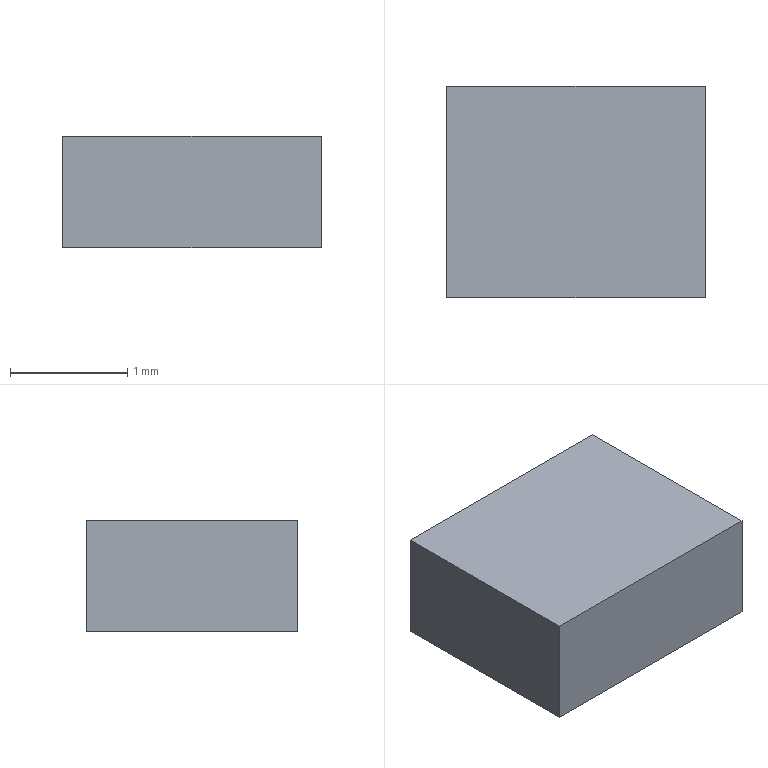Part | Creo | 1 solid | 6 faces | box 2.2 x 1.8 x 0.95 mm | volume 3.762 mm3 | plane 6
STEP:
#1=CARTESIAN_POINT('',(0.,0.,0.));
#2=DIRECTION('',(0.,0.,1.));
#3=DIRECTION('',(1.,0.,0.));
#4=AXIS2_PLACEMENT_3D('',#1,#2,#3);
#5=CARTESIAN_POINT('',(-1.1,0.9,0.));
#6=VERTEX_POINT('',#5);
#7=CARTESIAN_POINT('',(-1.1,-0.9,0.));
#8=VERTEX_POINT('',#7);
#9=CARTESIAN_POINT('',(-1.1,0.9,0.));
#10=DIRECTION('',(0.,-1.,0.));
#11=VECTOR('',#10,1.8);
#12=LINE('',#9,#11);
#13=EDGE_CURVE('',#6,#8,#12,.T.);
#14=ORIENTED_EDGE('',*,*,#13,.T.);
#15=CARTESIAN_POINT('',(1.1,-0.9,0.));
#16=VERTEX_POINT('',#15);
#17=CARTESIAN_POINT('',(-1.1,-0.9,0.));
#18=DIRECTION('',(1.,0.,0.));
#19=VECTOR('',#18,2.2);
#20=LINE('',#17,#19);
#21=EDGE_CURVE('',#8,#16,#20,.T.);
#22=ORIENTED_EDGE('',*,*,#21,.T.);
#23=CARTESIAN_POINT('',(1.1,0.9,0.));
#24=VERTEX_POINT('',#23);
#25=CARTESIAN_POINT('',(1.1,-0.9,0.));
#26=DIRECTION('',(0.,1.,0.));
#27=VECTOR('',#26,1.8);
#28=LINE('',#25,#27);
#29=EDGE_CURVE('',#16,#24,#28,.T.);
#30=ORIENTED_EDGE('',*,*,#29,.T.);
#31=CARTESIAN_POINT('',(1.1,0.9,0.));
#32=DIRECTION('',(-1.,0.,0.));
#33=VECTOR('',#32,2.2);
#34=LINE('',#31,#33);
#35=EDGE_CURVE('',#24,#6,#34,.T.);
#36=ORIENTED_EDGE('',*,*,#35,.T.);
#37=EDGE_LOOP('',(#14,#22,#30,#36));
#38=FACE_OUTER_BOUND('',#37,.F.);
#39=CARTESIAN_POINT('',(0.,0.,0.));
#40=DIRECTION('',(0.,0.,1.));
#41=DIRECTION('',(1.,0.,0.));
#42=AXIS2_PLACEMENT_3D('',#39,#40,#41);
#43=PLANE('',#42);
#44=ADVANCED_FACE('',(#38),#43,.F.);
#45=ORIENTED_EDGE('',*,*,#13,.F.);
#46=CARTESIAN_POINT('',(-1.1,0.9,0.95));
#47=VERTEX_POINT('',#46);
#48=CARTESIAN_POINT('',(-1.1,0.9,0.));
#49=DIRECTION('',(0.,0.,1.));
#50=VECTOR('',#49,0.95);
#51=LINE('',#48,#50);
#52=EDGE_CURVE('',#6,#47,#51,.T.);
#53=ORIENTED_EDGE('',*,*,#52,.T.);
#54=CARTESIAN_POINT('',(-1.1,-0.9,0.95));
#55=VERTEX_POINT('',#54);
#56=CARTESIAN_POINT('',(-1.1,0.9,0.95));
#57=DIRECTION('',(0.,-1.,0.));
#58=VECTOR('',#57,1.8);
#59=LINE('',#56,#58);
#60=EDGE_CURVE('',#47,#55,#59,.T.);
#61=ORIENTED_EDGE('',*,*,#60,.T.);
#62=CARTESIAN_POINT('',(-1.1,-0.9,0.));
#63=DIRECTION('',(0.,0.,1.));
#64=VECTOR('',#63,0.95);
#65=LINE('',#62,#64);
#66=EDGE_CURVE('',#8,#55,#65,.T.);
#67=ORIENTED_EDGE('',*,*,#66,.F.);
#68=EDGE_LOOP('',(#45,#53,#61,#67));
#69=FACE_OUTER_BOUND('',#68,.F.);
#70=CARTESIAN_POINT('',(-1.1,0.9,0.));
#71=DIRECTION('',(-1.,0.,0.));
#72=DIRECTION('',(0.,-1.,0.));
#73=AXIS2_PLACEMENT_3D('',#70,#71,#72);
#74=PLANE('',#73);
#75=ADVANCED_FACE('',(#69),#74,.T.);
#76=ORIENTED_EDGE('',*,*,#35,.F.);
#77=CARTESIAN_POINT('',(1.1,0.9,0.95));
#78=VERTEX_POINT('',#77);
#79=CARTESIAN_POINT('',(1.1,0.9,0.));
#80=DIRECTION('',(0.,0.,1.));
#81=VECTOR('',#80,0.95);
#82=LINE('',#79,#81);
#83=EDGE_CURVE('',#24,#78,#82,.T.);
#84=ORIENTED_EDGE('',*,*,#83,.T.);
#85=CARTESIAN_POINT('',(1.1,0.9,0.95));
#86=DIRECTION('',(-1.,0.,0.));
#87=VECTOR('',#86,2.2);
#88=LINE('',#85,#87);
#89=EDGE_CURVE('',#78,#47,#88,.T.);
#90=ORIENTED_EDGE('',*,*,#89,.T.);
#91=ORIENTED_EDGE('',*,*,#52,.F.);
#92=EDGE_LOOP('',(#76,#84,#90,#91));
#93=FACE_OUTER_BOUND('',#92,.F.);
#94=CARTESIAN_POINT('',(1.1,0.9,0.));
#95=DIRECTION('',(0.,1.,0.));
#96=DIRECTION('',(-1.,0.,0.));
#97=AXIS2_PLACEMENT_3D('',#94,#95,#96);
#98=PLANE('',#97);
#99=ADVANCED_FACE('',(#93),#98,.T.);
#100=ORIENTED_EDGE('',*,*,#29,.F.);
#101=CARTESIAN_POINT('',(1.1,-0.9,0.95));
#102=VERTEX_POINT('',#101);
#103=CARTESIAN_POINT('',(1.1,-0.9,0.));
#104=DIRECTION('',(0.,0.,1.));
#105=VECTOR('',#104,0.95);
#106=LINE('',#103,#105);
#107=EDGE_CURVE('',#16,#102,#106,.T.);
#108=ORIENTED_EDGE('',*,*,#107,.T.);
#109=CARTESIAN_POINT('',(1.1,-0.9,0.95));
#110=DIRECTION('',(0.,1.,0.));
#111=VECTOR('',#110,1.8);
#112=LINE('',#109,#111);
#113=EDGE_CURVE('',#102,#78,#112,.T.);
#114=ORIENTED_EDGE('',*,*,#113,.T.);
#115=ORIENTED_EDGE('',*,*,#83,.F.);
#116=EDGE_LOOP('',(#100,#108,#114,#115));
#117=FACE_OUTER_BOUND('',#116,.F.);
#118=CARTESIAN_POINT('',(1.1,-0.9,0.));
#119=DIRECTION('',(1.,0.,0.));
#120=DIRECTION('',(0.,1.,0.));
#121=AXIS2_PLACEMENT_3D('',#118,#119,#120);
#122=PLANE('',#121);
#123=ADVANCED_FACE('',(#117),#122,.T.);
#124=ORIENTED_EDGE('',*,*,#21,.F.);
#125=ORIENTED_EDGE('',*,*,#66,.T.);
#126=CARTESIAN_POINT('',(-1.1,-0.9,0.95));
#127=DIRECTION('',(1.,0.,0.));
#128=VECTOR('',#127,2.2);
#129=LINE('',#126,#128);
#130=EDGE_CURVE('',#55,#102,#129,.T.);
#131=ORIENTED_EDGE('',*,*,#130,.T.);
#132=ORIENTED_EDGE('',*,*,#107,.F.);
#133=EDGE_LOOP('',(#124,#125,#131,#132));
#134=FACE_OUTER_BOUND('',#133,.F.);
#135=CARTESIAN_POINT('',(-1.1,-0.9,0.));
#136=DIRECTION('',(0.,-1.,0.));
#137=DIRECTION('',(1.,0.,0.));
#138=AXIS2_PLACEMENT_3D('',#135,#136,#137);
#139=PLANE('',#138);
#140=ADVANCED_FACE('',(#134),#139,.T.);
#141=ORIENTED_EDGE('',*,*,#60,.F.);
#142=ORIENTED_EDGE('',*,*,#89,.F.);
#143=ORIENTED_EDGE('',*,*,#113,.F.);
#144=ORIENTED_EDGE('',*,*,#130,.F.);
#145=EDGE_LOOP('',(#141,#142,#143,#144));
#146=FACE_OUTER_BOUND('',#145,.F.);
#147=CARTESIAN_POINT('',(0.,0.,0.95));
#148=DIRECTION('',(0.,0.,1.));
#149=DIRECTION('',(1.,0.,0.));
#150=AXIS2_PLACEMENT_3D('',#147,#148,#149);
#151=PLANE('',#150);
#152=ADVANCED_FACE('',(#146),#151,.T.);
#153=CLOSED_SHELL('',(#44,#75,#99,#123,#140,#152));
#154=MANIFOLD_SOLID_BREP('',#153);
#155=(LENGTH_UNIT()NAMED_UNIT(*)SI_UNIT(.MILLI.,.METRE.));
#156=UNCERTAINTY_MEASURE_WITH_UNIT(LENGTH_MEASURE(0.0002997),#155,'','');
#157=(NAMED_UNIT(*)PLANE_ANGLE_UNIT()SI_UNIT($,.RADIAN.));
#158=PLANE_ANGLE_MEASURE_WITH_UNIT(PLANE_ANGLE_MEASURE(0.01745),#157);
#159=(CONVERSION_BASED_UNIT('DEGREE',#158)NAMED_UNIT(*)PLANE_ANGLE_UNIT());
#160=(NAMED_UNIT(*)SI_UNIT($,.STERADIAN.)SOLID_ANGLE_UNIT());
#161=(GEOMETRIC_REPRESENTATION_CONTEXT(3)GLOBAL_UNCERTAINTY_ASSIGNED_CONTEXT((#156))GLOBAL_UNIT_ASSIGNED_CONTEXT((#155,#159,#160))REPRESENTATION_CONTEXT('',''));
#162=ADVANCED_BREP_SHAPE_REPRESENTATION('',(#4,#154),#161);